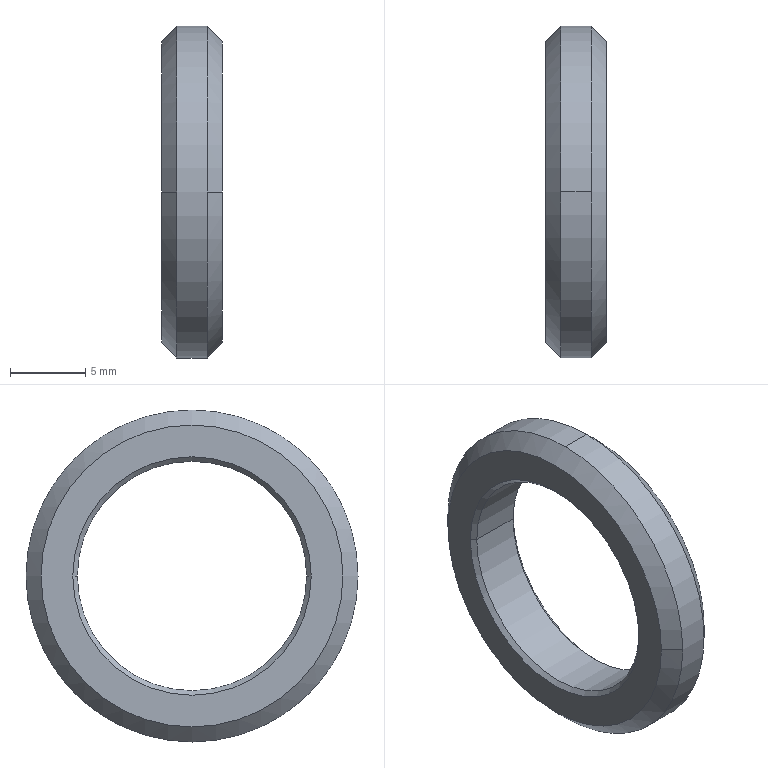Part | NX | 1 solid | 14 faces | box 4 x 22 x 22 mm | volume 723.322 mm3 | cone 8 | cylinder 4 | plane 2 | commonest cylinder face diameters 15.2 x2 22 x2
STEP:
#1=CARTESIAN_POINT('',(-141.,150.,-57.));
#2=VERTEX_POINT('',#1);
#3=CARTESIAN_POINT('',(-141.,161.,-46.));
#4=VERTEX_POINT('',#3);
#5=CARTESIAN_POINT('',(-141.,161.,-57.));
#6=DIRECTION('',(-1.,0.,0.));
#7=DIRECTION('',(0.,-1.,0.));
#8=AXIS2_PLACEMENT_3D('',#5,#6,#7);
#9=CIRCLE('',#8,11.);
#10=EDGE_CURVE('',#2,#4,#9,.T.);
#11=ORIENTED_EDGE('',*,*,#10,.T.);
#12=CARTESIAN_POINT('',(-143.,161.,-46.));
#13=VERTEX_POINT('',#12);
#14=CARTESIAN_POINT('',(-144.,161.,-46.));
#15=DIRECTION('',(-1.,0.,0.));
#16=VECTOR('',#15,1000.);
#17=LINE('',#14,#16);
#18=EDGE_CURVE('',#4,#13,#17,.T.);
#19=ORIENTED_EDGE('',*,*,#18,.T.);
#20=CARTESIAN_POINT('',(-143.,150.,-57.));
#21=VERTEX_POINT('',#20);
#22=CARTESIAN_POINT('',(-143.,161.,-57.));
#23=DIRECTION('',(-1.,0.,0.));
#24=DIRECTION('',(0.,-1.,0.));
#25=AXIS2_PLACEMENT_3D('',#22,#23,#24);
#26=CIRCLE('',#25,11.);
#27=EDGE_CURVE('',#21,#13,#26,.T.);
#28=ORIENTED_EDGE('',*,*,#27,.F.);
#29=CARTESIAN_POINT('',(-143.,161.,-68.));
#30=VERTEX_POINT('',#29);
#31=CARTESIAN_POINT('',(-143.,161.,-57.));
#32=DIRECTION('',(-1.,0.,0.));
#33=DIRECTION('',(0.,-1.,0.));
#34=AXIS2_PLACEMENT_3D('',#31,#32,#33);
#35=CIRCLE('',#34,11.);
#36=EDGE_CURVE('',#30,#21,#35,.T.);
#37=ORIENTED_EDGE('',*,*,#36,.F.);
#38=CARTESIAN_POINT('',(-141.,161.,-68.));
#39=VERTEX_POINT('',#38);
#40=CARTESIAN_POINT('',(-144.,161.,-68.));
#41=DIRECTION('',(-1.,0.,0.));
#42=VECTOR('',#41,1000.);
#43=LINE('',#40,#42);
#44=EDGE_CURVE('',#39,#30,#43,.T.);
#45=ORIENTED_EDGE('',*,*,#44,.F.);
#46=CARTESIAN_POINT('',(-141.,161.,-57.));
#47=DIRECTION('',(-1.,0.,0.));
#48=DIRECTION('',(0.,-1.,0.));
#49=AXIS2_PLACEMENT_3D('',#46,#47,#48);
#50=CIRCLE('',#49,11.);
#51=EDGE_CURVE('',#39,#2,#50,.T.);
#52=ORIENTED_EDGE('',*,*,#51,.T.);
#53=EDGE_LOOP('',(#11,#19,#28,#37,#45,#52));
#54=FACE_BOUND('',#53,.T.);
#55=CARTESIAN_POINT('',(-144.,161.,-57.));
#56=DIRECTION('',(-1.,0.,0.));
#57=DIRECTION('',(0.,0.,1.));
#58=AXIS2_PLACEMENT_3D('',#55,#56,#57);
#59=CYLINDRICAL_SURFACE('',#58,11.);
#60=ADVANCED_FACE('',(#54),#59,.T.);
#61=ORIENTED_EDGE('',*,*,#18,.F.);
#62=CARTESIAN_POINT('',(-141.,172.,-57.));
#63=VERTEX_POINT('',#62);
#64=CARTESIAN_POINT('',(-141.,161.,-57.));
#65=DIRECTION('',(-1.,0.,0.));
#66=DIRECTION('',(0.,-1.,0.));
#67=AXIS2_PLACEMENT_3D('',#64,#65,#66);
#68=CIRCLE('',#67,11.);
#69=EDGE_CURVE('',#4,#63,#68,.T.);
#70=ORIENTED_EDGE('',*,*,#69,.T.);
#71=CARTESIAN_POINT('',(-141.,161.,-57.));
#72=DIRECTION('',(-1.,0.,0.));
#73=DIRECTION('',(0.,-1.,0.));
#74=AXIS2_PLACEMENT_3D('',#71,#72,#73);
#75=CIRCLE('',#74,11.);
#76=EDGE_CURVE('',#63,#39,#75,.T.);
#77=ORIENTED_EDGE('',*,*,#76,.T.);
#78=ORIENTED_EDGE('',*,*,#44,.T.);
#79=CARTESIAN_POINT('',(-143.,172.,-57.));
#80=VERTEX_POINT('',#79);
#81=CARTESIAN_POINT('',(-143.,161.,-57.));
#82=DIRECTION('',(-1.,0.,0.));
#83=DIRECTION('',(0.,-1.,0.));
#84=AXIS2_PLACEMENT_3D('',#81,#82,#83);
#85=CIRCLE('',#84,11.);
#86=EDGE_CURVE('',#80,#30,#85,.T.);
#87=ORIENTED_EDGE('',*,*,#86,.F.);
#88=CARTESIAN_POINT('',(-143.,161.,-57.));
#89=DIRECTION('',(-1.,0.,0.));
#90=DIRECTION('',(0.,-1.,0.));
#91=AXIS2_PLACEMENT_3D('',#88,#89,#90);
#92=CIRCLE('',#91,11.);
#93=EDGE_CURVE('',#13,#80,#92,.T.);
#94=ORIENTED_EDGE('',*,*,#93,.F.);
#95=EDGE_LOOP('',(#61,#70,#77,#78,#87,#94));
#96=FACE_BOUND('',#95,.T.);
#97=CARTESIAN_POINT('',(-144.,161.,-57.));
#98=DIRECTION('',(-1.,0.,0.));
#99=DIRECTION('',(0.,0.,1.));
#100=AXIS2_PLACEMENT_3D('',#97,#98,#99);
#101=CYLINDRICAL_SURFACE('',#100,11.);
#102=ADVANCED_FACE('',(#96),#101,.T.);
#103=CARTESIAN_POINT('',(-140.3,168.6,-57.));
#104=VERTEX_POINT('',#103);
#105=CARTESIAN_POINT('',(-140.3,153.4,-57.));
#106=VERTEX_POINT('',#105);
#107=CARTESIAN_POINT('',(-140.3,161.,-57.));
#108=DIRECTION('',(-1.,0.,0.));
#109=DIRECTION('',(0.,-1.,0.));
#110=AXIS2_PLACEMENT_3D('',#107,#108,#109);
#111=CIRCLE('',#110,7.6);
#112=EDGE_CURVE('',#104,#106,#111,.T.);
#113=ORIENTED_EDGE('',*,*,#112,.F.);
#114=CARTESIAN_POINT('',(-143.7,168.6,-57.));
#115=VERTEX_POINT('',#114);
#116=CARTESIAN_POINT('',(-144.,168.6,-57.));
#117=DIRECTION('',(-1.,0.,0.));
#118=VECTOR('',#117,1000.);
#119=LINE('',#116,#118);
#120=EDGE_CURVE('',#115,#104,#119,.F.);
#121=ORIENTED_EDGE('',*,*,#120,.F.);
#122=CARTESIAN_POINT('',(-143.7,153.4,-57.));
#123=VERTEX_POINT('',#122);
#124=CARTESIAN_POINT('',(-143.7,161.,-57.));
#125=DIRECTION('',(-1.,0.,0.));
#126=DIRECTION('',(0.,-1.,0.));
#127=AXIS2_PLACEMENT_3D('',#124,#125,#126);
#128=CIRCLE('',#127,7.6);
#129=EDGE_CURVE('',#115,#123,#128,.T.);
#130=ORIENTED_EDGE('',*,*,#129,.T.);
#131=CARTESIAN_POINT('',(-144.,153.4,-57.));
#132=DIRECTION('',(-1.,0.,0.));
#133=VECTOR('',#132,1000.);
#134=LINE('',#131,#133);
#135=EDGE_CURVE('',#123,#106,#134,.F.);
#136=ORIENTED_EDGE('',*,*,#135,.T.);
#137=EDGE_LOOP('',(#113,#121,#130,#136));
#138=FACE_BOUND('',#137,.T.);
#139=CARTESIAN_POINT('',(-144.,161.,-57.));
#140=DIRECTION('',(-1.,0.,0.));
#141=DIRECTION('',(0.,-1.,0.));
#142=AXIS2_PLACEMENT_3D('',#139,#140,#141);
#143=CYLINDRICAL_SURFACE('',#142,7.6);
#144=ADVANCED_FACE('',(#138),#143,.F.);
#145=ORIENTED_EDGE('',*,*,#135,.F.);
#146=CARTESIAN_POINT('',(-143.7,161.,-57.));
#147=DIRECTION('',(-1.,0.,0.));
#148=DIRECTION('',(0.,-1.,0.));
#149=AXIS2_PLACEMENT_3D('',#146,#147,#148);
#150=CIRCLE('',#149,7.6);
#151=EDGE_CURVE('',#123,#115,#150,.T.);
#152=ORIENTED_EDGE('',*,*,#151,.T.);
#153=ORIENTED_EDGE('',*,*,#120,.T.);
#154=CARTESIAN_POINT('',(-140.3,161.,-57.));
#155=DIRECTION('',(-1.,0.,0.));
#156=DIRECTION('',(0.,-1.,0.));
#157=AXIS2_PLACEMENT_3D('',#154,#155,#156);
#158=CIRCLE('',#157,7.6);
#159=EDGE_CURVE('',#106,#104,#158,.T.);
#160=ORIENTED_EDGE('',*,*,#159,.F.);
#161=EDGE_LOOP('',(#145,#152,#153,#160));
#162=FACE_BOUND('',#161,.T.);
#163=CARTESIAN_POINT('',(-144.,161.,-57.));
#164=DIRECTION('',(-1.,0.,0.));
#165=DIRECTION('',(0.,-1.,0.));
#166=AXIS2_PLACEMENT_3D('',#163,#164,#165);
#167=CYLINDRICAL_SURFACE('',#166,7.6);
#168=ADVANCED_FACE('',(#162),#167,.F.);
#169=CARTESIAN_POINT('',(-140.,151.,-57.));
#170=VERTEX_POINT('',#169);
#171=CARTESIAN_POINT('',(-140.,171.,-57.));
#172=VERTEX_POINT('',#171);
#173=CARTESIAN_POINT('',(-140.,161.,-57.));
#174=DIRECTION('',(-1.,0.,0.));
#175=DIRECTION('',(0.,-1.,0.));
#176=AXIS2_PLACEMENT_3D('',#173,#174,#175);
#177=CIRCLE('',#176,10.);
#178=EDGE_CURVE('',#170,#172,#177,.T.);
#179=ORIENTED_EDGE('',*,*,#178,.F.);
#180=CARTESIAN_POINT('',(-140.,161.,-57.));
#181=DIRECTION('',(-1.,0.,0.));
#182=DIRECTION('',(0.,-1.,0.));
#183=AXIS2_PLACEMENT_3D('',#180,#181,#182);
#184=CIRCLE('',#183,10.);
#185=EDGE_CURVE('',#172,#170,#184,.T.);
#186=ORIENTED_EDGE('',*,*,#185,.F.);
#187=EDGE_LOOP('',(#179,#186));
#188=FACE_BOUND('',#187,.T.);
#189=CARTESIAN_POINT('',(-140.,168.9,-57.));
#190=VERTEX_POINT('',#189);
#191=CARTESIAN_POINT('',(-140.,153.1,-57.));
#192=VERTEX_POINT('',#191);
#193=CARTESIAN_POINT('',(-140.,161.,-57.));
#194=DIRECTION('',(-1.,0.,0.));
#195=DIRECTION('',(0.,-1.,0.));
#196=AXIS2_PLACEMENT_3D('',#193,#194,#195);
#197=CIRCLE('',#196,7.9);
#198=EDGE_CURVE('',#190,#192,#197,.T.);
#199=ORIENTED_EDGE('',*,*,#198,.T.);
#200=CARTESIAN_POINT('',(-140.,161.,-57.));
#201=DIRECTION('',(-1.,0.,0.));
#202=DIRECTION('',(0.,-1.,0.));
#203=AXIS2_PLACEMENT_3D('',#200,#201,#202);
#204=CIRCLE('',#203,7.9);
#205=EDGE_CURVE('',#192,#190,#204,.T.);
#206=ORIENTED_EDGE('',*,*,#205,.T.);
#207=EDGE_LOOP('',(#199,#206));
#208=FACE_BOUND('',#207,.T.);
#209=CARTESIAN_POINT('',(-140.,171.479,-46.149));
#210=DIRECTION('',(1.,0.,0.));
#211=DIRECTION('',(0.,-1.,0.));
#212=AXIS2_PLACEMENT_3D('',#209,#210,#211);
#213=PLANE('',#212);
#214=ADVANCED_FACE('',(#188,#208),#213,.T.);
#215=ORIENTED_EDGE('',*,*,#178,.T.);
#216=CARTESIAN_POINT('',(-140.,171.,-57.));
#217=DIRECTION('',(-0.7071,0.7071,0.));
#218=VECTOR('',#217,1000.);
#219=LINE('',#216,#218);
#220=EDGE_CURVE('',#172,#63,#219,.T.);
#221=ORIENTED_EDGE('',*,*,#220,.T.);
#222=ORIENTED_EDGE('',*,*,#69,.F.);
#223=ORIENTED_EDGE('',*,*,#10,.F.);
#224=CARTESIAN_POINT('',(-140.,151.,-57.));
#225=DIRECTION('',(-0.7071,-0.7071,0.));
#226=VECTOR('',#225,1000.);
#227=LINE('',#224,#226);
#228=EDGE_CURVE('',#170,#2,#227,.T.);
#229=ORIENTED_EDGE('',*,*,#228,.F.);
#230=EDGE_LOOP('',(#215,#221,#222,#223,#229));
#231=FACE_BOUND('',#230,.T.);
#232=CARTESIAN_POINT('',(-140.,161.,-57.));
#233=DIRECTION('',(-1.,0.,0.));
#234=DIRECTION('',(0.,-1.,0.));
#235=AXIS2_PLACEMENT_3D('',#232,#233,#234);
#236=CONICAL_SURFACE('',#235,10.,0.7854);
#237=ADVANCED_FACE('',(#231),#236,.T.);
#238=ORIENTED_EDGE('',*,*,#198,.F.);
#239=CARTESIAN_POINT('',(-140.,168.9,-57.));
#240=DIRECTION('',(0.7071,0.7071,0.));
#241=VECTOR('',#240,1000.);
#242=LINE('',#239,#241);
#243=EDGE_CURVE('',#104,#190,#242,.T.);
#244=ORIENTED_EDGE('',*,*,#243,.F.);
#245=ORIENTED_EDGE('',*,*,#112,.T.);
#246=CARTESIAN_POINT('',(-140.,153.1,-57.));
#247=DIRECTION('',(0.7071,-0.7071,0.));
#248=VECTOR('',#247,1000.);
#249=LINE('',#246,#248);
#250=EDGE_CURVE('',#106,#192,#249,.T.);
#251=ORIENTED_EDGE('',*,*,#250,.T.);
#252=EDGE_LOOP('',(#238,#244,#245,#251));
#253=FACE_BOUND('',#252,.T.);
#254=CARTESIAN_POINT('',(-140.,161.,-57.));
#255=DIRECTION('',(1.,0.,0.));
#256=DIRECTION('',(0.,1.,0.));
#257=AXIS2_PLACEMENT_3D('',#254,#255,#256);
#258=CONICAL_SURFACE('',#257,7.9,0.7854);
#259=ADVANCED_FACE('',(#253),#258,.F.);
#260=ORIENTED_EDGE('',*,*,#243,.T.);
#261=ORIENTED_EDGE('',*,*,#205,.F.);
#262=ORIENTED_EDGE('',*,*,#250,.F.);
#263=ORIENTED_EDGE('',*,*,#159,.T.);
#264=EDGE_LOOP('',(#260,#261,#262,#263));
#265=FACE_BOUND('',#264,.T.);
#266=CARTESIAN_POINT('',(-140.,161.,-57.));
#267=DIRECTION('',(1.,0.,0.));
#268=DIRECTION('',(0.,1.,0.));
#269=AXIS2_PLACEMENT_3D('',#266,#267,#268);
#270=CONICAL_SURFACE('',#269,7.9,0.7854);
#271=ADVANCED_FACE('',(#265),#270,.F.);
#272=ORIENTED_EDGE('',*,*,#220,.F.);
#273=ORIENTED_EDGE('',*,*,#185,.T.);
#274=ORIENTED_EDGE('',*,*,#228,.T.);
#275=ORIENTED_EDGE('',*,*,#51,.F.);
#276=ORIENTED_EDGE('',*,*,#76,.F.);
#277=EDGE_LOOP('',(#272,#273,#274,#275,#276));
#278=FACE_BOUND('',#277,.T.);
#279=CARTESIAN_POINT('',(-140.,161.,-57.));
#280=DIRECTION('',(-1.,0.,0.));
#281=DIRECTION('',(0.,-1.,0.));
#282=AXIS2_PLACEMENT_3D('',#279,#280,#281);
#283=CONICAL_SURFACE('',#282,10.,0.7854);
#284=ADVANCED_FACE('',(#278),#283,.T.);
#285=CARTESIAN_POINT('',(-144.,151.,-57.));
#286=VERTEX_POINT('',#285);
#287=CARTESIAN_POINT('',(-144.,171.,-57.));
#288=VERTEX_POINT('',#287);
#289=CARTESIAN_POINT('',(-144.,161.,-57.));
#290=DIRECTION('',(-1.,0.,0.));
#291=DIRECTION('',(0.,-1.,0.));
#292=AXIS2_PLACEMENT_3D('',#289,#290,#291);
#293=CIRCLE('',#292,10.);
#294=EDGE_CURVE('',#286,#288,#293,.T.);
#295=ORIENTED_EDGE('',*,*,#294,.T.);
#296=CARTESIAN_POINT('',(-144.,161.,-57.));
#297=DIRECTION('',(-1.,0.,0.));
#298=DIRECTION('',(0.,-1.,0.));
#299=AXIS2_PLACEMENT_3D('',#296,#297,#298);
#300=CIRCLE('',#299,10.);
#301=EDGE_CURVE('',#288,#286,#300,.T.);
#302=ORIENTED_EDGE('',*,*,#301,.T.);
#303=EDGE_LOOP('',(#295,#302));
#304=FACE_BOUND('',#303,.T.);
#305=CARTESIAN_POINT('',(-144.,168.9,-57.));
#306=VERTEX_POINT('',#305);
#307=CARTESIAN_POINT('',(-144.,153.1,-57.));
#308=VERTEX_POINT('',#307);
#309=CARTESIAN_POINT('',(-144.,161.,-57.));
#310=DIRECTION('',(-1.,0.,0.));
#311=DIRECTION('',(0.,-1.,0.));
#312=AXIS2_PLACEMENT_3D('',#309,#310,#311);
#313=CIRCLE('',#312,7.9);
#314=EDGE_CURVE('',#306,#308,#313,.T.);
#315=ORIENTED_EDGE('',*,*,#314,.F.);
#316=CARTESIAN_POINT('',(-144.,161.,-57.));
#317=DIRECTION('',(-1.,0.,0.));
#318=DIRECTION('',(0.,-1.,0.));
#319=AXIS2_PLACEMENT_3D('',#316,#317,#318);
#320=CIRCLE('',#319,7.9);
#321=EDGE_CURVE('',#308,#306,#320,.T.);
#322=ORIENTED_EDGE('',*,*,#321,.F.);
#323=EDGE_LOOP('',(#315,#322));
#324=FACE_BOUND('',#323,.T.);
#325=CARTESIAN_POINT('',(-144.,171.479,-46.149));
#326=DIRECTION('',(1.,0.,0.));
#327=DIRECTION('',(0.,-1.,0.));
#328=AXIS2_PLACEMENT_3D('',#325,#326,#327);
#329=PLANE('',#328);
#330=ADVANCED_FACE('',(#304,#324),#329,.F.);
#331=ORIENTED_EDGE('',*,*,#294,.F.);
#332=CARTESIAN_POINT('',(-144.,151.,-57.));
#333=DIRECTION('',(0.7071,-0.7071,0.));
#334=VECTOR('',#333,1000.);
#335=LINE('',#332,#334);
#336=EDGE_CURVE('',#21,#286,#335,.F.);
#337=ORIENTED_EDGE('',*,*,#336,.F.);
#338=ORIENTED_EDGE('',*,*,#27,.T.);
#339=ORIENTED_EDGE('',*,*,#93,.T.);
#340=CARTESIAN_POINT('',(-144.,171.,-57.));
#341=DIRECTION('',(0.7071,0.7071,0.));
#342=VECTOR('',#341,1000.);
#343=LINE('',#340,#342);
#344=EDGE_CURVE('',#80,#288,#343,.F.);
#345=ORIENTED_EDGE('',*,*,#344,.T.);
#346=EDGE_LOOP('',(#331,#337,#338,#339,#345));
#347=FACE_BOUND('',#346,.T.);
#348=CARTESIAN_POINT('',(-144.,161.,-57.));
#349=DIRECTION('',(1.,0.,0.));
#350=DIRECTION('',(0.,1.,0.));
#351=AXIS2_PLACEMENT_3D('',#348,#349,#350);
#352=CONICAL_SURFACE('',#351,10.,0.7854);
#353=ADVANCED_FACE('',(#347),#352,.T.);
#354=ORIENTED_EDGE('',*,*,#314,.T.);
#355=CARTESIAN_POINT('',(-144.,153.1,-57.));
#356=DIRECTION('',(-0.7071,-0.7071,0.));
#357=VECTOR('',#356,1000.);
#358=LINE('',#355,#357);
#359=EDGE_CURVE('',#308,#123,#358,.F.);
#360=ORIENTED_EDGE('',*,*,#359,.T.);
#361=ORIENTED_EDGE('',*,*,#129,.F.);
#362=CARTESIAN_POINT('',(-144.,168.9,-57.));
#363=DIRECTION('',(-0.7071,0.7071,0.));
#364=VECTOR('',#363,1000.);
#365=LINE('',#362,#364);
#366=EDGE_CURVE('',#306,#115,#365,.F.);
#367=ORIENTED_EDGE('',*,*,#366,.F.);
#368=EDGE_LOOP('',(#354,#360,#361,#367));
#369=FACE_BOUND('',#368,.T.);
#370=CARTESIAN_POINT('',(-144.,161.,-57.));
#371=DIRECTION('',(-1.,0.,0.));
#372=DIRECTION('',(0.,-1.,0.));
#373=AXIS2_PLACEMENT_3D('',#370,#371,#372);
#374=CONICAL_SURFACE('',#373,7.9,0.7854);
#375=ADVANCED_FACE('',(#369),#374,.F.);
#376=ORIENTED_EDGE('',*,*,#336,.T.);
#377=ORIENTED_EDGE('',*,*,#301,.F.);
#378=ORIENTED_EDGE('',*,*,#344,.F.);
#379=ORIENTED_EDGE('',*,*,#86,.T.);
#380=ORIENTED_EDGE('',*,*,#36,.T.);
#381=EDGE_LOOP('',(#376,#377,#378,#379,#380));
#382=FACE_BOUND('',#381,.T.);
#383=CARTESIAN_POINT('',(-144.,161.,-57.));
#384=DIRECTION('',(1.,0.,0.));
#385=DIRECTION('',(0.,1.,0.));
#386=AXIS2_PLACEMENT_3D('',#383,#384,#385);
#387=CONICAL_SURFACE('',#386,10.,0.7854);
#388=ADVANCED_FACE('',(#382),#387,.T.);
#389=ORIENTED_EDGE('',*,*,#359,.F.);
#390=ORIENTED_EDGE('',*,*,#321,.T.);
#391=ORIENTED_EDGE('',*,*,#366,.T.);
#392=ORIENTED_EDGE('',*,*,#151,.F.);
#393=EDGE_LOOP('',(#389,#390,#391,#392));
#394=FACE_BOUND('',#393,.T.);
#395=CARTESIAN_POINT('',(-144.,161.,-57.));
#396=DIRECTION('',(-1.,0.,0.));
#397=DIRECTION('',(0.,-1.,0.));
#398=AXIS2_PLACEMENT_3D('',#395,#396,#397);
#399=CONICAL_SURFACE('',#398,7.9,0.7854);
#400=ADVANCED_FACE('',(#394),#399,.F.);
#401=CLOSED_SHELL('',(#60,#102,#144,#168,#214,#237,#259,#271,#284,#330,#353,#375,#388,#400));
#402=MANIFOLD_SOLID_BREP('',#401);
#403=(LENGTH_UNIT()NAMED_UNIT(*)SI_UNIT(.MILLI.,.METRE.));
#404=UNCERTAINTY_MEASURE_WITH_UNIT(LENGTH_MEASURE(0.00001),#403,'','');
#405=(NAMED_UNIT(*)PLANE_ANGLE_UNIT()SI_UNIT($,.RADIAN.));
#406=(NAMED_UNIT(*)SI_UNIT($,.STERADIAN.)SOLID_ANGLE_UNIT());
#407=(GEOMETRIC_REPRESENTATION_CONTEXT(3)GLOBAL_UNCERTAINTY_ASSIGNED_CONTEXT((#404))GLOBAL_UNIT_ASSIGNED_CONTEXT((#403,#405,#406))REPRESENTATION_CONTEXT('',''));
#408=ADVANCED_BREP_SHAPE_REPRESENTATION('',(#402),#407);